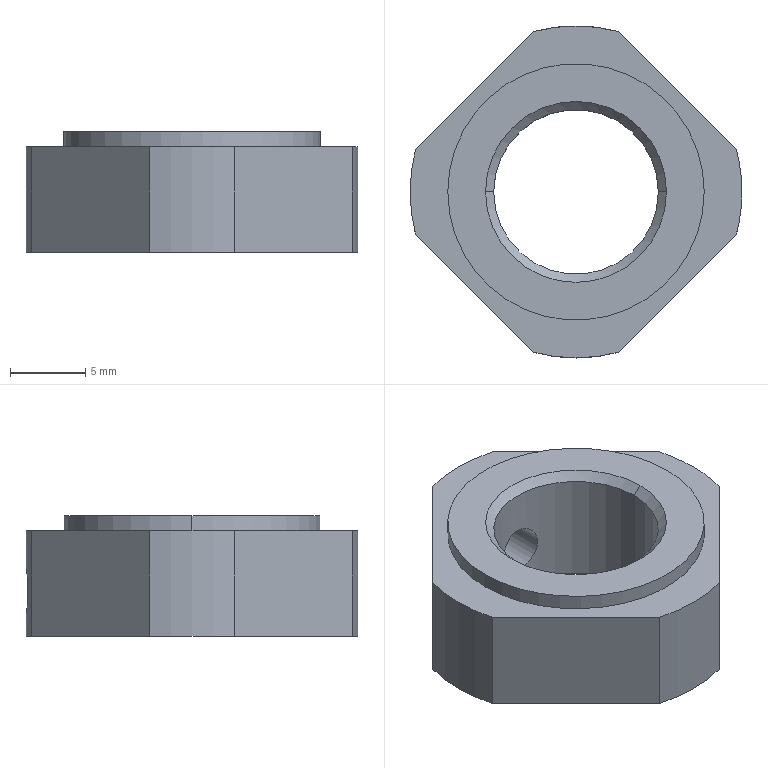Part | STEP file | Locking bearing nut BKN21-M12 (M12×1.0)_yhda | 1 solid | 20 faces | box 22 x 22 x 8 mm | volume 1773 mm3 | cylinder 11 | plane 7 | cone 2 | commonest cylinder face diameters 22 x5 3.242 x2 10.917 x2 17 x2